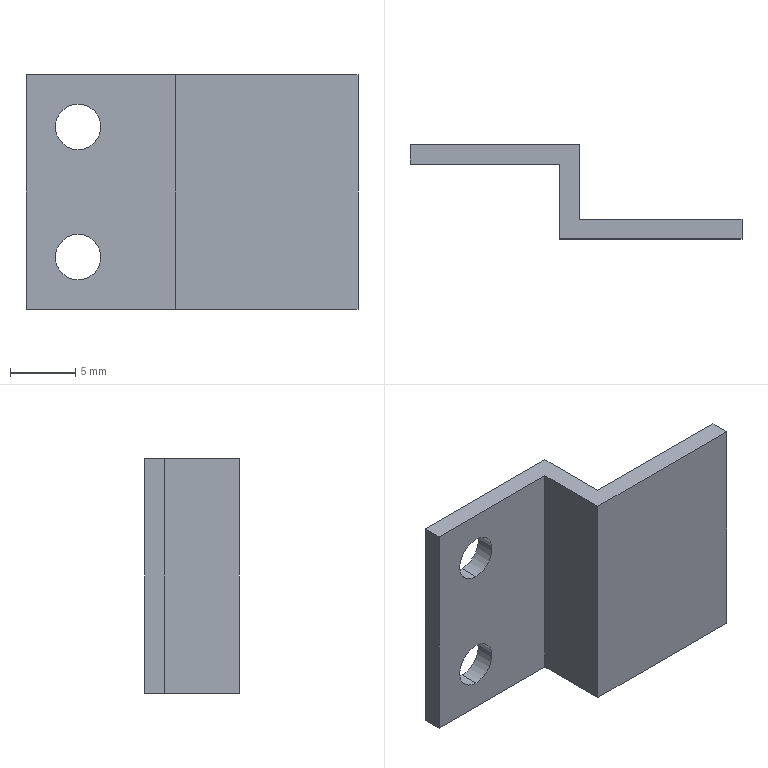Part | STEP file | SM140A-20-1140D-140A-600 External sensor plate | 1 solid | 14 faces | box 25.5 x 7.25 x 18 mm | volume 814.887 mm3 | plane 10 | cylinder 4 | commonest cylinder face diameters 3.5 x4
STEP:
#1=CARTESIAN_POINT('',(0.,0.,0.));
#2=DIRECTION('',(0.,0.,1.));
#3=DIRECTION('',(1.,0.,0.));
#4=AXIS2_PLACEMENT_3D('',#1,#2,#3);
#5=CARTESIAN_POINT('',(4.,-1.5,5.75));
#6=VERTEX_POINT('',#5);
#7=CARTESIAN_POINT('',(4.,0.,5.75));
#8=VERTEX_POINT('',#7);
#9=CARTESIAN_POINT('',(4.,-7.25,5.75));
#10=DIRECTION('',(0.,1.,0.));
#11=VECTOR('',#10,1.);
#12=LINE('',#9,#11);
#13=CARTESIAN_POINT('',(4.,-7.25,4.));
#14=DIRECTION('',(0.,1.,0.));
#15=DIRECTION('',(0.,0.,1.));
#16=AXIS2_PLACEMENT_3D('',#13,#14,#15);
#17=CYLINDRICAL_SURFACE('',#16,1.75);
#18=CARTESIAN_POINT('',(6.283,0.));
#19=DIRECTION('',(0.,1.));
#20=VECTOR('',#19,1.);
#21=LINE('',#18,#20);
#22=(GEOMETRIC_REPRESENTATION_CONTEXT(2)PARAMETRIC_REPRESENTATION_CONTEXT()REPRESENTATION_CONTEXT('',''));
#23=DEFINITIONAL_REPRESENTATION('',(#21),#22);
#24=PCURVE('',#17,#23);
#25=CARTESIAN_POINT('',(4.,-7.25,4.));
#26=DIRECTION('',(0.,1.,0.));
#27=DIRECTION('',(0.,0.,1.));
#28=AXIS2_PLACEMENT_3D('',#25,#26,#27);
#29=CYLINDRICAL_SURFACE('',#28,1.75);
#30=CARTESIAN_POINT('',(0.,0.));
#31=DIRECTION('',(0.,1.));
#32=VECTOR('',#31,1.);
#33=LINE('',#30,#32);
#34=(GEOMETRIC_REPRESENTATION_CONTEXT(2)PARAMETRIC_REPRESENTATION_CONTEXT()REPRESENTATION_CONTEXT('',''));
#35=DEFINITIONAL_REPRESENTATION('',(#33),#34);
#36=PCURVE('',#29,#35);
#37=SURFACE_CURVE('',#12,(#24,#36),.PCURVE_S1.);
#38=EDGE_CURVE('',#6,#8,#37,.T.);
#39=ORIENTED_EDGE('',*,*,#38,.T.);
#40=CARTESIAN_POINT('',(4.,0.,2.25));
#41=VERTEX_POINT('',#40);
#42=CARTESIAN_POINT('',(4.,0.,4.));
#43=DIRECTION('',(0.,1.,0.));
#44=DIRECTION('',(0.,0.,1.));
#45=AXIS2_PLACEMENT_3D('',#42,#43,#44);
#46=CIRCLE('',#45,1.75);
#47=CARTESIAN_POINT('',(0.,7.25));
#48=DIRECTION('',(1.,0.));
#49=VECTOR('',#48,1.);
#50=LINE('',#47,#49);
#51=(GEOMETRIC_REPRESENTATION_CONTEXT(2)PARAMETRIC_REPRESENTATION_CONTEXT()REPRESENTATION_CONTEXT('',''));
#52=DEFINITIONAL_REPRESENTATION('',(#50),#51);
#53=PCURVE('',#17,#52);
#54=CARTESIAN_POINT('',(0.,0.,18.));
#55=DIRECTION('',(0.,-1.,0.));
#56=DIRECTION('',(0.,0.,-1.));
#57=AXIS2_PLACEMENT_3D('',#54,#55,#56);
#58=PLANE('',#57);
#59=CARTESIAN_POINT('',(12.25,4.));
#60=CARTESIAN_POINT('',(12.25,7.031));
#61=CARTESIAN_POINT('',(14.875,5.516));
#62=CARTESIAN_POINT('',(17.5,4.));
#63=CARTESIAN_POINT('',(14.875,2.484));
#64=CARTESIAN_POINT('',(12.25,0.9689));
#65=CARTESIAN_POINT('',(12.25,4.));
#66=(BOUNDED_CURVE()B_SPLINE_CURVE(2,(#59,#60,#61,#62,#63,#64,#65),.UNSPECIFIED.,.T.,.F.)B_SPLINE_CURVE_WITH_KNOTS((1,2,2,2,2,1),(-2.094,0.,2.094,4.189,6.283,8.378),.UNSPECIFIED.)CURVE()GEOMETRIC_REPRESENTATION_ITEM()RATIONAL_B_SPLINE_CURVE((1.,0.5,1.,0.5,1.,0.5,1.))REPRESENTATION_ITEM(''));
#67=(GEOMETRIC_REPRESENTATION_CONTEXT(2)PARAMETRIC_REPRESENTATION_CONTEXT()REPRESENTATION_CONTEXT('',''));
#68=DEFINITIONAL_REPRESENTATION('',(#66),#67);
#69=PCURVE('',#58,#68);
#70=SURFACE_CURVE('',#46,(#53,#69),.PCURVE_S1.);
#71=EDGE_CURVE('',#41,#8,#70,.T.);
#72=ORIENTED_EDGE('',*,*,#71,.F.);
#73=CARTESIAN_POINT('',(4.,-1.5,2.25));
#74=VERTEX_POINT('',#73);
#75=CARTESIAN_POINT('',(4.,-7.25,2.25));
#76=DIRECTION('',(0.,1.,0.));
#77=VECTOR('',#76,1.);
#78=LINE('',#75,#77);
#79=CARTESIAN_POINT('',(3.142,0.));
#80=DIRECTION('',(0.,1.));
#81=VECTOR('',#80,1.);
#82=LINE('',#79,#81);
#83=(GEOMETRIC_REPRESENTATION_CONTEXT(2)PARAMETRIC_REPRESENTATION_CONTEXT()REPRESENTATION_CONTEXT('',''));
#84=DEFINITIONAL_REPRESENTATION('',(#82),#83);
#85=PCURVE('',#17,#84);
#86=CARTESIAN_POINT('',(3.142,0.));
#87=DIRECTION('',(0.,1.));
#88=VECTOR('',#87,1.);
#89=LINE('',#86,#88);
#90=(GEOMETRIC_REPRESENTATION_CONTEXT(2)PARAMETRIC_REPRESENTATION_CONTEXT()REPRESENTATION_CONTEXT('',''));
#91=DEFINITIONAL_REPRESENTATION('',(#89),#90);
#92=PCURVE('',#29,#91);
#93=SURFACE_CURVE('',#78,(#85,#92),.PCURVE_S1.);
#94=EDGE_CURVE('',#74,#41,#93,.T.);
#95=ORIENTED_EDGE('',*,*,#94,.F.);
#96=CARTESIAN_POINT('',(4.,-1.5,4.));
#97=DIRECTION('',(0.,1.,0.));
#98=DIRECTION('',(-1.,0.,0.));
#99=AXIS2_PLACEMENT_3D('',#96,#97,#98);
#100=CIRCLE('',#99,1.75);
#101=CARTESIAN_POINT('',(-1.571,5.75));
#102=DIRECTION('',(1.,0.));
#103=VECTOR('',#102,1.);
#104=LINE('',#101,#103);
#105=(GEOMETRIC_REPRESENTATION_CONTEXT(2)PARAMETRIC_REPRESENTATION_CONTEXT()REPRESENTATION_CONTEXT('',''));
#106=DEFINITIONAL_REPRESENTATION('',(#104),#105);
#107=PCURVE('',#17,#106);
#108=CARTESIAN_POINT('',(11.5,-1.5,18.));
#109=DIRECTION('',(0.,1.,0.));
#110=DIRECTION('',(-1.,0.,0.));
#111=AXIS2_PLACEMENT_3D('',#108,#109,#110);
#112=PLANE('',#111);
#113=CARTESIAN_POINT('',(7.5,-14.));
#114=DIRECTION('',(1.,0.));
#115=AXIS2_PLACEMENT_2D('',#113,#114);
#116=CIRCLE('',#115,1.75);
#117=(GEOMETRIC_REPRESENTATION_CONTEXT(2)PARAMETRIC_REPRESENTATION_CONTEXT()REPRESENTATION_CONTEXT('',''));
#118=DEFINITIONAL_REPRESENTATION('',(#116),#117);
#119=PCURVE('',#112,#118);
#120=SURFACE_CURVE('',#100,(#107,#119),.PCURVE_S1.);
#121=EDGE_CURVE('',#74,#6,#120,.T.);
#122=ORIENTED_EDGE('',*,*,#121,.T.);
#123=EDGE_LOOP('',(#39,#72,#95,#122));
#124=FACE_BOUND('',#123,.F.);
#125=ADVANCED_FACE('',(#124),#17,.F.);
#126=CARTESIAN_POINT('',(4.,-1.5,15.75));
#127=VERTEX_POINT('',#126);
#128=CARTESIAN_POINT('',(4.,0.,15.75));
#129=VERTEX_POINT('',#128);
#130=CARTESIAN_POINT('',(4.,-7.25,15.75));
#131=DIRECTION('',(0.,1.,0.));
#132=VECTOR('',#131,1.);
#133=LINE('',#130,#132);
#134=CARTESIAN_POINT('',(4.,-7.25,14.));
#135=DIRECTION('',(0.,1.,0.));
#136=DIRECTION('',(0.,0.,1.));
#137=AXIS2_PLACEMENT_3D('',#134,#135,#136);
#138=CYLINDRICAL_SURFACE('',#137,1.75);
#139=CARTESIAN_POINT('',(6.283,0.));
#140=DIRECTION('',(0.,1.));
#141=VECTOR('',#140,1.);
#142=LINE('',#139,#141);
#143=(GEOMETRIC_REPRESENTATION_CONTEXT(2)PARAMETRIC_REPRESENTATION_CONTEXT()REPRESENTATION_CONTEXT('',''));
#144=DEFINITIONAL_REPRESENTATION('',(#142),#143);
#145=PCURVE('',#138,#144);
#146=CARTESIAN_POINT('',(4.,-7.25,14.));
#147=DIRECTION('',(0.,1.,0.));
#148=DIRECTION('',(0.,0.,1.));
#149=AXIS2_PLACEMENT_3D('',#146,#147,#148);
#150=CYLINDRICAL_SURFACE('',#149,1.75);
#151=CARTESIAN_POINT('',(0.,0.));
#152=DIRECTION('',(0.,1.));
#153=VECTOR('',#152,1.);
#154=LINE('',#151,#153);
#155=(GEOMETRIC_REPRESENTATION_CONTEXT(2)PARAMETRIC_REPRESENTATION_CONTEXT()REPRESENTATION_CONTEXT('',''));
#156=DEFINITIONAL_REPRESENTATION('',(#154),#155);
#157=PCURVE('',#150,#156);
#158=SURFACE_CURVE('',#133,(#145,#157),.PCURVE_S1.);
#159=EDGE_CURVE('',#127,#129,#158,.T.);
#160=ORIENTED_EDGE('',*,*,#159,.T.);
#161=CARTESIAN_POINT('',(4.,0.,12.25));
#162=VERTEX_POINT('',#161);
#163=CARTESIAN_POINT('',(4.,0.,14.));
#164=DIRECTION('',(0.,1.,0.));
#165=DIRECTION('',(0.,0.,1.));
#166=AXIS2_PLACEMENT_3D('',#163,#164,#165);
#167=CIRCLE('',#166,1.75);
#168=CARTESIAN_POINT('',(0.,7.25));
#169=DIRECTION('',(1.,0.));
#170=VECTOR('',#169,1.);
#171=LINE('',#168,#170);
#172=(GEOMETRIC_REPRESENTATION_CONTEXT(2)PARAMETRIC_REPRESENTATION_CONTEXT()REPRESENTATION_CONTEXT('',''));
#173=DEFINITIONAL_REPRESENTATION('',(#171),#172);
#174=PCURVE('',#138,#173);
#175=CARTESIAN_POINT('',(2.25,4.));
#176=CARTESIAN_POINT('',(2.25,7.031));
#177=CARTESIAN_POINT('',(4.875,5.516));
#178=CARTESIAN_POINT('',(7.5,4.));
#179=CARTESIAN_POINT('',(4.875,2.484));
#180=CARTESIAN_POINT('',(2.25,0.9689));
#181=CARTESIAN_POINT('',(2.25,4.));
#182=(BOUNDED_CURVE()B_SPLINE_CURVE(2,(#175,#176,#177,#178,#179,#180,#181),.UNSPECIFIED.,.T.,.F.)B_SPLINE_CURVE_WITH_KNOTS((1,2,2,2,2,1),(-2.094,0.,2.094,4.189,6.283,8.378),.UNSPECIFIED.)CURVE()GEOMETRIC_REPRESENTATION_ITEM()RATIONAL_B_SPLINE_CURVE((1.,0.5,1.,0.5,1.,0.5,1.))REPRESENTATION_ITEM(''));
#183=(GEOMETRIC_REPRESENTATION_CONTEXT(2)PARAMETRIC_REPRESENTATION_CONTEXT()REPRESENTATION_CONTEXT('',''));
#184=DEFINITIONAL_REPRESENTATION('',(#182),#183);
#185=PCURVE('',#58,#184);
#186=SURFACE_CURVE('',#167,(#174,#185),.PCURVE_S1.);
#187=EDGE_CURVE('',#162,#129,#186,.T.);
#188=ORIENTED_EDGE('',*,*,#187,.F.);
#189=CARTESIAN_POINT('',(4.,-1.5,12.25));
#190=VERTEX_POINT('',#189);
#191=CARTESIAN_POINT('',(4.,-7.25,12.25));
#192=DIRECTION('',(0.,1.,0.));
#193=VECTOR('',#192,1.);
#194=LINE('',#191,#193);
#195=CARTESIAN_POINT('',(3.142,0.));
#196=DIRECTION('',(0.,1.));
#197=VECTOR('',#196,1.);
#198=LINE('',#195,#197);
#199=(GEOMETRIC_REPRESENTATION_CONTEXT(2)PARAMETRIC_REPRESENTATION_CONTEXT()REPRESENTATION_CONTEXT('',''));
#200=DEFINITIONAL_REPRESENTATION('',(#198),#199);
#201=PCURVE('',#138,#200);
#202=CARTESIAN_POINT('',(3.142,0.));
#203=DIRECTION('',(0.,1.));
#204=VECTOR('',#203,1.);
#205=LINE('',#202,#204);
#206=(GEOMETRIC_REPRESENTATION_CONTEXT(2)PARAMETRIC_REPRESENTATION_CONTEXT()REPRESENTATION_CONTEXT('',''));
#207=DEFINITIONAL_REPRESENTATION('',(#205),#206);
#208=PCURVE('',#150,#207);
#209=SURFACE_CURVE('',#194,(#201,#208),.PCURVE_S1.);
#210=EDGE_CURVE('',#190,#162,#209,.T.);
#211=ORIENTED_EDGE('',*,*,#210,.F.);
#212=CARTESIAN_POINT('',(4.,-1.5,14.));
#213=DIRECTION('',(0.,1.,0.));
#214=DIRECTION('',(-1.,0.,0.));
#215=AXIS2_PLACEMENT_3D('',#212,#213,#214);
#216=CIRCLE('',#215,1.75);
#217=CARTESIAN_POINT('',(-1.571,5.75));
#218=DIRECTION('',(1.,0.));
#219=VECTOR('',#218,1.);
#220=LINE('',#217,#219);
#221=(GEOMETRIC_REPRESENTATION_CONTEXT(2)PARAMETRIC_REPRESENTATION_CONTEXT()REPRESENTATION_CONTEXT('',''));
#222=DEFINITIONAL_REPRESENTATION('',(#220),#221);
#223=PCURVE('',#138,#222);
#224=CARTESIAN_POINT('',(7.5,-4.));
#225=DIRECTION('',(1.,0.));
#226=AXIS2_PLACEMENT_2D('',#224,#225);
#227=CIRCLE('',#226,1.75);
#228=(GEOMETRIC_REPRESENTATION_CONTEXT(2)PARAMETRIC_REPRESENTATION_CONTEXT()REPRESENTATION_CONTEXT('',''));
#229=DEFINITIONAL_REPRESENTATION('',(#227),#228);
#230=PCURVE('',#112,#229);
#231=SURFACE_CURVE('',#216,(#223,#230),.PCURVE_S1.);
#232=EDGE_CURVE('',#190,#127,#231,.T.);
#233=ORIENTED_EDGE('',*,*,#232,.T.);
#234=EDGE_LOOP('',(#160,#188,#211,#233));
#235=FACE_BOUND('',#234,.F.);
#236=ADVANCED_FACE('',(#235),#138,.F.);
#237=CARTESIAN_POINT('',(0.,0.,0.));
#238=VERTEX_POINT('',#237);
#239=CARTESIAN_POINT('',(0.,-1.5,0.));
#240=VERTEX_POINT('',#239);
#241=CARTESIAN_POINT('',(0.,-1.5,0.));
#242=DIRECTION('',(0.,-1.,0.));
#243=VECTOR('',#242,1.);
#244=LINE('',#241,#243);
#245=CARTESIAN_POINT('',(0.,-1.5,18.));
#246=DIRECTION('',(1.,0.,0.));
#247=DIRECTION('',(0.,0.,-1.));
#248=AXIS2_PLACEMENT_3D('',#245,#246,#247);
#249=PLANE('',#248);
#250=CARTESIAN_POINT('',(18.,0.));
#251=DIRECTION('',(0.,-1.));
#252=VECTOR('',#251,1.);
#253=LINE('',#250,#252);
#254=(GEOMETRIC_REPRESENTATION_CONTEXT(2)PARAMETRIC_REPRESENTATION_CONTEXT()REPRESENTATION_CONTEXT('',''));
#255=DEFINITIONAL_REPRESENTATION('',(#253),#254);
#256=PCURVE('',#249,#255);
#257=CARTESIAN_POINT('',(0.,0.,0.));
#258=DIRECTION('',(0.,0.,-1.));
#259=DIRECTION('',(-1.,0.,0.));
#260=AXIS2_PLACEMENT_3D('',#257,#258,#259);
#261=PLANE('',#260);
#262=CARTESIAN_POINT('',(0.,-1.5));
#263=DIRECTION('',(0.,-1.));
#264=VECTOR('',#263,1.);
#265=LINE('',#262,#264);
#266=(GEOMETRIC_REPRESENTATION_CONTEXT(2)PARAMETRIC_REPRESENTATION_CONTEXT()REPRESENTATION_CONTEXT('',''));
#267=DEFINITIONAL_REPRESENTATION('',(#265),#266);
#268=PCURVE('',#261,#267);
#269=SURFACE_CURVE('',#244,(#256,#268),.PCURVE_S1.);
#270=EDGE_CURVE('',#238,#240,#269,.T.);
#271=ORIENTED_EDGE('',*,*,#270,.T.);
#272=CARTESIAN_POINT('',(0.,-1.5,18.));
#273=VERTEX_POINT('',#272);
#274=CARTESIAN_POINT('',(0.,-1.5,18.));
#275=DIRECTION('',(0.,0.,-1.));
#276=VECTOR('',#275,1.);
#277=LINE('',#274,#276);
#278=CARTESIAN_POINT('',(0.,0.));
#279=DIRECTION('',(1.,0.));
#280=VECTOR('',#279,1.);
#281=LINE('',#278,#280);
#282=(GEOMETRIC_REPRESENTATION_CONTEXT(2)PARAMETRIC_REPRESENTATION_CONTEXT()REPRESENTATION_CONTEXT('',''));
#283=DEFINITIONAL_REPRESENTATION('',(#281),#282);
#284=PCURVE('',#249,#283);
#285=CARTESIAN_POINT('',(11.5,0.));
#286=DIRECTION('',(0.,-1.));
#287=VECTOR('',#286,1.);
#288=LINE('',#285,#287);
#289=(GEOMETRIC_REPRESENTATION_CONTEXT(2)PARAMETRIC_REPRESENTATION_CONTEXT()REPRESENTATION_CONTEXT('',''));
#290=DEFINITIONAL_REPRESENTATION('',(#288),#289);
#291=PCURVE('',#112,#290);
#292=SURFACE_CURVE('',#277,(#284,#291),.PCURVE_S1.);
#293=EDGE_CURVE('',#273,#240,#292,.T.);
#294=ORIENTED_EDGE('',*,*,#293,.F.);
#295=CARTESIAN_POINT('',(0.,0.,18.));
#296=VERTEX_POINT('',#295);
#297=CARTESIAN_POINT('',(0.,-1.5,18.));
#298=DIRECTION('',(0.,-1.,0.));
#299=VECTOR('',#298,1.);
#300=LINE('',#297,#299);
#301=CARTESIAN_POINT('',(0.,0.));
#302=DIRECTION('',(0.,-1.));
#303=VECTOR('',#302,1.);
#304=LINE('',#301,#303);
#305=(GEOMETRIC_REPRESENTATION_CONTEXT(2)PARAMETRIC_REPRESENTATION_CONTEXT()REPRESENTATION_CONTEXT('',''));
#306=DEFINITIONAL_REPRESENTATION('',(#304),#305);
#307=PCURVE('',#249,#306);
#308=CARTESIAN_POINT('',(0.,0.,18.));
#309=DIRECTION('',(0.,0.,-1.));
#310=DIRECTION('',(-1.,0.,0.));
#311=AXIS2_PLACEMENT_3D('',#308,#309,#310);
#312=PLANE('',#311);
#313=CARTESIAN_POINT('',(0.,-1.5));
#314=DIRECTION('',(0.,-1.));
#315=VECTOR('',#314,1.);
#316=LINE('',#313,#315);
#317=(GEOMETRIC_REPRESENTATION_CONTEXT(2)PARAMETRIC_REPRESENTATION_CONTEXT()REPRESENTATION_CONTEXT('',''));
#318=DEFINITIONAL_REPRESENTATION('',(#316),#317);
#319=PCURVE('',#312,#318);
#320=SURFACE_CURVE('',#300,(#307,#319),.PCURVE_S1.);
#321=EDGE_CURVE('',#296,#273,#320,.T.);
#322=ORIENTED_EDGE('',*,*,#321,.F.);
#323=CARTESIAN_POINT('',(0.,0.,18.));
#324=DIRECTION('',(0.,0.,-1.));
#325=VECTOR('',#324,1.);
#326=LINE('',#323,#325);
#327=CARTESIAN_POINT('',(0.,1.5));
#328=DIRECTION('',(1.,0.));
#329=VECTOR('',#328,1.);
#330=LINE('',#327,#329);
#331=(GEOMETRIC_REPRESENTATION_CONTEXT(2)PARAMETRIC_REPRESENTATION_CONTEXT()REPRESENTATION_CONTEXT('',''));
#332=DEFINITIONAL_REPRESENTATION('',(#330),#331);
#333=PCURVE('',#249,#332);
#334=CARTESIAN_POINT('',(0.,0.));
#335=DIRECTION('',(1.,0.));
#336=VECTOR('',#335,1.);
#337=LINE('',#334,#336);
#338=(GEOMETRIC_REPRESENTATION_CONTEXT(2)PARAMETRIC_REPRESENTATION_CONTEXT()REPRESENTATION_CONTEXT('',''));
#339=DEFINITIONAL_REPRESENTATION('',(#337),#338);
#340=PCURVE('',#58,#339);
#341=SURFACE_CURVE('',#326,(#333,#340),.PCURVE_S1.);
#342=EDGE_CURVE('',#296,#238,#341,.T.);
#343=ORIENTED_EDGE('',*,*,#342,.T.);
#344=EDGE_LOOP('',(#271,#294,#322,#343));
#345=FACE_BOUND('',#344,.T.);
#346=ADVANCED_FACE('',(#345),#249,.F.);
#347=CARTESIAN_POINT('',(4.,-1.5,4.));
#348=DIRECTION('',(0.,1.,0.));
#349=DIRECTION('',(-1.,0.,0.));
#350=AXIS2_PLACEMENT_3D('',#347,#348,#349);
#351=CIRCLE('',#350,1.75);
#352=CARTESIAN_POINT('',(7.5,-14.));
#353=DIRECTION('',(1.,0.));
#354=AXIS2_PLACEMENT_2D('',#352,#353);
#355=CIRCLE('',#354,1.75);
#356=(GEOMETRIC_REPRESENTATION_CONTEXT(2)PARAMETRIC_REPRESENTATION_CONTEXT()REPRESENTATION_CONTEXT('',''));
#357=DEFINITIONAL_REPRESENTATION('',(#355),#356);
#358=PCURVE('',#112,#357);
#359=CARTESIAN_POINT('',(-1.571,5.75));
#360=DIRECTION('',(1.,0.));
#361=VECTOR('',#360,1.);
#362=LINE('',#359,#361);
#363=(GEOMETRIC_REPRESENTATION_CONTEXT(2)PARAMETRIC_REPRESENTATION_CONTEXT()REPRESENTATION_CONTEXT('',''));
#364=DEFINITIONAL_REPRESENTATION('',(#362),#363);
#365=PCURVE('',#29,#364);
#366=SURFACE_CURVE('',#351,(#358,#365),.PCURVE_S1.);
#367=EDGE_CURVE('',#6,#74,#366,.T.);
#368=ORIENTED_EDGE('',*,*,#367,.T.);
#369=ORIENTED_EDGE('',*,*,#121,.T.);
#370=EDGE_LOOP('',(#368,#369));
#371=FACE_BOUND('',#370,.T.);
#372=CARTESIAN_POINT('',(4.,-1.5,14.));
#373=DIRECTION('',(0.,1.,0.));
#374=DIRECTION('',(-1.,0.,0.));
#375=AXIS2_PLACEMENT_3D('',#372,#373,#374);
#376=CIRCLE('',#375,1.75);
#377=CARTESIAN_POINT('',(7.5,-4.));
#378=DIRECTION('',(1.,0.));
#379=AXIS2_PLACEMENT_2D('',#377,#378);
#380=CIRCLE('',#379,1.75);
#381=(GEOMETRIC_REPRESENTATION_CONTEXT(2)PARAMETRIC_REPRESENTATION_CONTEXT()REPRESENTATION_CONTEXT('',''));
#382=DEFINITIONAL_REPRESENTATION('',(#380),#381);
#383=PCURVE('',#112,#382);
#384=CARTESIAN_POINT('',(-1.571,5.75));
#385=DIRECTION('',(1.,0.));
#386=VECTOR('',#385,1.);
#387=LINE('',#384,#386);
#388=(GEOMETRIC_REPRESENTATION_CONTEXT(2)PARAMETRIC_REPRESENTATION_CONTEXT()REPRESENTATION_CONTEXT('',''));
#389=DEFINITIONAL_REPRESENTATION('',(#387),#388);
#390=PCURVE('',#150,#389);
#391=SURFACE_CURVE('',#376,(#383,#390),.PCURVE_S1.);
#392=EDGE_CURVE('',#127,#190,#391,.T.);
#393=ORIENTED_EDGE('',*,*,#392,.T.);
#394=ORIENTED_EDGE('',*,*,#232,.T.);
#395=EDGE_LOOP('',(#393,#394));
#396=FACE_BOUND('',#395,.T.);
#397=CARTESIAN_POINT('',(11.5,-1.5,0.));
#398=VERTEX_POINT('',#397);
#399=CARTESIAN_POINT('',(11.5,-1.5,0.));
#400=DIRECTION('',(1.,0.,0.));
#401=VECTOR('',#400,1.);
#402=LINE('',#399,#401);
#403=CARTESIAN_POINT('',(0.,-18.));
#404=DIRECTION('',(-1.,0.));
#405=VECTOR('',#404,1.);
#406=LINE('',#403,#405);
#407=(GEOMETRIC_REPRESENTATION_CONTEXT(2)PARAMETRIC_REPRESENTATION_CONTEXT()REPRESENTATION_CONTEXT('',''));
#408=DEFINITIONAL_REPRESENTATION('',(#406),#407);
#409=PCURVE('',#112,#408);
#410=CARTESIAN_POINT('',(-11.5,-1.5));
#411=DIRECTION('',(-1.,0.));
#412=VECTOR('',#411,1.);
#413=LINE('',#410,#412);
#414=(GEOMETRIC_REPRESENTATION_CONTEXT(2)PARAMETRIC_REPRESENTATION_CONTEXT()REPRESENTATION_CONTEXT('',''));
#415=DEFINITIONAL_REPRESENTATION('',(#413),#414);
#416=PCURVE('',#261,#415);
#417=SURFACE_CURVE('',#402,(#409,#416),.PCURVE_S1.);
#418=EDGE_CURVE('',#240,#398,#417,.T.);
#419=ORIENTED_EDGE('',*,*,#418,.T.);
#420=CARTESIAN_POINT('',(11.5,-1.5,18.));
#421=VERTEX_POINT('',#420);
#422=CARTESIAN_POINT('',(11.5,-1.5,18.));
#423=DIRECTION('',(0.,0.,-1.));
#424=VECTOR('',#423,1.);
#425=LINE('',#422,#424);
#426=CARTESIAN_POINT('',(0.,0.));
#427=DIRECTION('',(0.,-1.));
#428=VECTOR('',#427,1.);
#429=LINE('',#426,#428);
#430=(GEOMETRIC_REPRESENTATION_CONTEXT(2)PARAMETRIC_REPRESENTATION_CONTEXT()REPRESENTATION_CONTEXT('',''));
#431=DEFINITIONAL_REPRESENTATION('',(#429),#430);
#432=PCURVE('',#112,#431);
#433=CARTESIAN_POINT('',(11.5,-7.25,18.));
#434=DIRECTION('',(1.,0.,0.));
#435=DIRECTION('',(0.,0.,-1.));
#436=AXIS2_PLACEMENT_3D('',#433,#434,#435);
#437=PLANE('',#436);
#438=CARTESIAN_POINT('',(0.,5.75));
#439=DIRECTION('',(1.,0.));
#440=VECTOR('',#439,1.);
#441=LINE('',#438,#440);
#442=(GEOMETRIC_REPRESENTATION_CONTEXT(2)PARAMETRIC_REPRESENTATION_CONTEXT()REPRESENTATION_CONTEXT('',''));
#443=DEFINITIONAL_REPRESENTATION('',(#441),#442);
#444=PCURVE('',#437,#443);
#445=SURFACE_CURVE('',#425,(#432,#444),.PCURVE_S1.);
#446=EDGE_CURVE('',#421,#398,#445,.T.);
#447=ORIENTED_EDGE('',*,*,#446,.F.);
#448=CARTESIAN_POINT('',(11.5,-1.5,18.));
#449=DIRECTION('',(1.,0.,0.));
#450=VECTOR('',#449,1.);
#451=LINE('',#448,#450);
#452=CARTESIAN_POINT('',(0.,0.));
#453=DIRECTION('',(-1.,0.));
#454=VECTOR('',#453,1.);
#455=LINE('',#452,#454);
#456=(GEOMETRIC_REPRESENTATION_CONTEXT(2)PARAMETRIC_REPRESENTATION_CONTEXT()REPRESENTATION_CONTEXT('',''));
#457=DEFINITIONAL_REPRESENTATION('',(#455),#456);
#458=PCURVE('',#112,#457);
#459=CARTESIAN_POINT('',(-11.5,-1.5));
#460=DIRECTION('',(-1.,0.));
#461=VECTOR('',#460,1.);
#462=LINE('',#459,#461);
#463=(GEOMETRIC_REPRESENTATION_CONTEXT(2)PARAMETRIC_REPRESENTATION_CONTEXT()REPRESENTATION_CONTEXT('',''));
#464=DEFINITIONAL_REPRESENTATION('',(#462),#463);
#465=PCURVE('',#312,#464);
#466=SURFACE_CURVE('',#451,(#458,#465),.PCURVE_S1.);
#467=EDGE_CURVE('',#273,#421,#466,.T.);
#468=ORIENTED_EDGE('',*,*,#467,.F.);
#469=ORIENTED_EDGE('',*,*,#293,.T.);
#470=EDGE_LOOP('',(#419,#447,#468,#469));
#471=FACE_BOUND('',#470,.T.);
#472=ADVANCED_FACE('',(#371,#396,#471),#112,.F.);
#473=CARTESIAN_POINT('',(11.5,-7.25,0.));
#474=VERTEX_POINT('',#473);
#475=CARTESIAN_POINT('',(11.5,-7.25,0.));
#476=DIRECTION('',(0.,-1.,0.));
#477=VECTOR('',#476,1.);
#478=LINE('',#475,#477);
#479=CARTESIAN_POINT('',(18.,0.));
#480=DIRECTION('',(0.,-1.));
#481=VECTOR('',#480,1.);
#482=LINE('',#479,#481);
#483=(GEOMETRIC_REPRESENTATION_CONTEXT(2)PARAMETRIC_REPRESENTATION_CONTEXT()REPRESENTATION_CONTEXT('',''));
#484=DEFINITIONAL_REPRESENTATION('',(#482),#483);
#485=PCURVE('',#437,#484);
#486=CARTESIAN_POINT('',(-11.5,-7.25));
#487=DIRECTION('',(0.,-1.));
#488=VECTOR('',#487,1.);
#489=LINE('',#486,#488);
#490=(GEOMETRIC_REPRESENTATION_CONTEXT(2)PARAMETRIC_REPRESENTATION_CONTEXT()REPRESENTATION_CONTEXT('',''));
#491=DEFINITIONAL_REPRESENTATION('',(#489),#490);
#492=PCURVE('',#261,#491);
#493=SURFACE_CURVE('',#478,(#485,#492),.PCURVE_S1.);
#494=EDGE_CURVE('',#398,#474,#493,.T.);
#495=ORIENTED_EDGE('',*,*,#494,.T.);
#496=CARTESIAN_POINT('',(11.5,-7.25,18.));
#497=VERTEX_POINT('',#496);
#498=CARTESIAN_POINT('',(11.5,-7.25,18.));
#499=DIRECTION('',(0.,0.,-1.));
#500=VECTOR('',#499,1.);
#501=LINE('',#498,#500);
#502=CARTESIAN_POINT('',(0.,0.));
#503=DIRECTION('',(1.,0.));
#504=VECTOR('',#503,1.);
#505=LINE('',#502,#504);
#506=(GEOMETRIC_REPRESENTATION_CONTEXT(2)PARAMETRIC_REPRESENTATION_CONTEXT()REPRESENTATION_CONTEXT('',''));
#507=DEFINITIONAL_REPRESENTATION('',(#505),#506);
#508=PCURVE('',#437,#507);
#509=CARTESIAN_POINT('',(25.5,-7.25,18.));
#510=DIRECTION('',(0.,1.,0.));
#511=DIRECTION('',(-1.,0.,0.));
#512=AXIS2_PLACEMENT_3D('',#509,#510,#511);
#513=PLANE('',#512);
#514=CARTESIAN_POINT('',(14.,0.));
#515=DIRECTION('',(0.,-1.));
#516=VECTOR('',#515,1.);
#517=LINE('',#514,#516);
#518=(GEOMETRIC_REPRESENTATION_CONTEXT(2)PARAMETRIC_REPRESENTATION_CONTEXT()REPRESENTATION_CONTEXT('',''));
#519=DEFINITIONAL_REPRESENTATION('',(#517),#518);
#520=PCURVE('',#513,#519);
#521=SURFACE_CURVE('',#501,(#508,#520),.PCURVE_S1.);
#522=EDGE_CURVE('',#497,#474,#521,.T.);
#523=ORIENTED_EDGE('',*,*,#522,.F.);
#524=CARTESIAN_POINT('',(11.5,-7.25,18.));
#525=DIRECTION('',(0.,-1.,0.));
#526=VECTOR('',#525,1.);
#527=LINE('',#524,#526);
#528=CARTESIAN_POINT('',(0.,0.));
#529=DIRECTION('',(0.,-1.));
#530=VECTOR('',#529,1.);
#531=LINE('',#528,#530);
#532=(GEOMETRIC_REPRESENTATION_CONTEXT(2)PARAMETRIC_REPRESENTATION_CONTEXT()REPRESENTATION_CONTEXT('',''));
#533=DEFINITIONAL_REPRESENTATION('',(#531),#532);
#534=PCURVE('',#437,#533);
#535=CARTESIAN_POINT('',(-11.5,-7.25));
#536=DIRECTION('',(0.,-1.));
#537=VECTOR('',#536,1.);
#538=LINE('',#535,#537);
#539=(GEOMETRIC_REPRESENTATION_CONTEXT(2)PARAMETRIC_REPRESENTATION_CONTEXT()REPRESENTATION_CONTEXT('',''));
#540=DEFINITIONAL_REPRESENTATION('',(#538),#539);
#541=PCURVE('',#312,#540);
#542=SURFACE_CURVE('',#527,(#534,#541),.PCURVE_S1.);
#543=EDGE_CURVE('',#421,#497,#542,.T.);
#544=ORIENTED_EDGE('',*,*,#543,.F.);
#545=ORIENTED_EDGE('',*,*,#446,.T.);
#546=EDGE_LOOP('',(#495,#523,#544,#545));
#547=FACE_BOUND('',#546,.T.);
#548=ADVANCED_FACE('',(#547),#437,.F.);
#549=CARTESIAN_POINT('',(25.5,-7.25,0.));
#550=VERTEX_POINT('',#549);
#551=CARTESIAN_POINT('',(25.5,-7.25,0.));
#552=DIRECTION('',(1.,0.,0.));
#553=VECTOR('',#552,1.);
#554=LINE('',#551,#553);
#555=CARTESIAN_POINT('',(0.,-18.));
#556=DIRECTION('',(-1.,0.));
#557=VECTOR('',#556,1.);
#558=LINE('',#555,#557);
#559=(GEOMETRIC_REPRESENTATION_CONTEXT(2)PARAMETRIC_REPRESENTATION_CONTEXT()REPRESENTATION_CONTEXT('',''));
#560=DEFINITIONAL_REPRESENTATION('',(#558),#559);
#561=PCURVE('',#513,#560);
#562=CARTESIAN_POINT('',(-25.5,-7.25));
#563=DIRECTION('',(-1.,0.));
#564=VECTOR('',#563,1.);
#565=LINE('',#562,#564);
#566=(GEOMETRIC_REPRESENTATION_CONTEXT(2)PARAMETRIC_REPRESENTATION_CONTEXT()REPRESENTATION_CONTEXT('',''));
#567=DEFINITIONAL_REPRESENTATION('',(#565),#566);
#568=PCURVE('',#261,#567);
#569=SURFACE_CURVE('',#554,(#561,#568),.PCURVE_S1.);
#570=EDGE_CURVE('',#474,#550,#569,.T.);
#571=ORIENTED_EDGE('',*,*,#570,.T.);
#572=CARTESIAN_POINT('',(25.5,-7.25,18.));
#573=VERTEX_POINT('',#572);
#574=CARTESIAN_POINT('',(25.5,-7.25,18.));
#575=DIRECTION('',(0.,0.,-1.));
#576=VECTOR('',#575,1.);
#577=LINE('',#574,#576);
#578=CARTESIAN_POINT('',(0.,0.));
#579=DIRECTION('',(0.,-1.));
#580=VECTOR('',#579,1.);
#581=LINE('',#578,#580);
#582=(GEOMETRIC_REPRESENTATION_CONTEXT(2)PARAMETRIC_REPRESENTATION_CONTEXT()REPRESENTATION_CONTEXT('',''));
#583=DEFINITIONAL_REPRESENTATION('',(#581),#582);
#584=PCURVE('',#513,#583);
#585=CARTESIAN_POINT('',(25.5,-5.75,18.));
#586=DIRECTION('',(-1.,0.,0.));
#587=DIRECTION('',(0.,0.,1.));
#588=AXIS2_PLACEMENT_3D('',#585,#586,#587);
#589=PLANE('',#588);
#590=CARTESIAN_POINT('',(0.,-1.5));
#591=DIRECTION('',(-1.,0.));
#592=VECTOR('',#591,1.);
#593=LINE('',#590,#592);
#594=(GEOMETRIC_REPRESENTATION_CONTEXT(2)PARAMETRIC_REPRESENTATION_CONTEXT()REPRESENTATION_CONTEXT('',''));
#595=DEFINITIONAL_REPRESENTATION('',(#593),#594);
#596=PCURVE('',#589,#595);
#597=SURFACE_CURVE('',#577,(#584,#596),.PCURVE_S1.);
#598=EDGE_CURVE('',#573,#550,#597,.T.);
#599=ORIENTED_EDGE('',*,*,#598,.F.);
#600=CARTESIAN_POINT('',(25.5,-7.25,18.));
#601=DIRECTION('',(1.,0.,0.));
#602=VECTOR('',#601,1.);
#603=LINE('',#600,#602);
#604=CARTESIAN_POINT('',(0.,0.));
#605=DIRECTION('',(-1.,0.));
#606=VECTOR('',#605,1.);
#607=LINE('',#604,#606);
#608=(GEOMETRIC_REPRESENTATION_CONTEXT(2)PARAMETRIC_REPRESENTATION_CONTEXT()REPRESENTATION_CONTEXT('',''));
#609=DEFINITIONAL_REPRESENTATION('',(#607),#608);
#610=PCURVE('',#513,#609);
#611=CARTESIAN_POINT('',(-25.5,-7.25));
#612=DIRECTION('',(-1.,0.));
#613=VECTOR('',#612,1.);
#614=LINE('',#611,#613);
#615=(GEOMETRIC_REPRESENTATION_CONTEXT(2)PARAMETRIC_REPRESENTATION_CONTEXT()REPRESENTATION_CONTEXT('',''));
#616=DEFINITIONAL_REPRESENTATION('',(#614),#615);
#617=PCURVE('',#312,#616);
#618=SURFACE_CURVE('',#603,(#610,#617),.PCURVE_S1.);
#619=EDGE_CURVE('',#497,#573,#618,.T.);
#620=ORIENTED_EDGE('',*,*,#619,.F.);
#621=ORIENTED_EDGE('',*,*,#522,.T.);
#622=EDGE_LOOP('',(#571,#599,#620,#621));
#623=FACE_BOUND('',#622,.T.);
#624=ADVANCED_FACE('',(#623),#513,.F.);
#625=CARTESIAN_POINT('',(25.5,-5.75,0.));
#626=VERTEX_POINT('',#625);
#627=CARTESIAN_POINT('',(25.5,-5.75,0.));
#628=DIRECTION('',(0.,1.,0.));
#629=VECTOR('',#628,1.);
#630=LINE('',#627,#629);
#631=CARTESIAN_POINT('',(-18.,0.));
#632=DIRECTION('',(0.,1.));
#633=VECTOR('',#632,1.);
#634=LINE('',#631,#633);
#635=(GEOMETRIC_REPRESENTATION_CONTEXT(2)PARAMETRIC_REPRESENTATION_CONTEXT()REPRESENTATION_CONTEXT('',''));
#636=DEFINITIONAL_REPRESENTATION('',(#634),#635);
#637=PCURVE('',#589,#636);
#638=CARTESIAN_POINT('',(-25.5,-5.75));
#639=DIRECTION('',(0.,1.));
#640=VECTOR('',#639,1.);
#641=LINE('',#638,#640);
#642=(GEOMETRIC_REPRESENTATION_CONTEXT(2)PARAMETRIC_REPRESENTATION_CONTEXT()REPRESENTATION_CONTEXT('',''));
#643=DEFINITIONAL_REPRESENTATION('',(#641),#642);
#644=PCURVE('',#261,#643);
#645=SURFACE_CURVE('',#630,(#637,#644),.PCURVE_S1.);
#646=EDGE_CURVE('',#550,#626,#645,.T.);
#647=ORIENTED_EDGE('',*,*,#646,.T.);
#648=CARTESIAN_POINT('',(25.5,-5.75,18.));
#649=VERTEX_POINT('',#648);
#650=CARTESIAN_POINT('',(25.5,-5.75,18.));
#651=DIRECTION('',(0.,0.,-1.));
#652=VECTOR('',#651,1.);
#653=LINE('',#650,#652);
#654=CARTESIAN_POINT('',(0.,0.));
#655=DIRECTION('',(-1.,0.));
#656=VECTOR('',#655,1.);
#657=LINE('',#654,#656);
#658=(GEOMETRIC_REPRESENTATION_CONTEXT(2)PARAMETRIC_REPRESENTATION_CONTEXT()REPRESENTATION_CONTEXT('',''));
#659=DEFINITIONAL_REPRESENTATION('',(#657),#658);
#660=PCURVE('',#589,#659);
#661=CARTESIAN_POINT('',(13.,-5.75,18.));
#662=DIRECTION('',(0.,-1.,0.));
#663=DIRECTION('',(0.,0.,-1.));
#664=AXIS2_PLACEMENT_3D('',#661,#662,#663);
#665=PLANE('',#664);
#666=CARTESIAN_POINT('',(0.,12.5));
#667=DIRECTION('',(1.,0.));
#668=VECTOR('',#667,1.);
#669=LINE('',#666,#668);
#670=(GEOMETRIC_REPRESENTATION_CONTEXT(2)PARAMETRIC_REPRESENTATION_CONTEXT()REPRESENTATION_CONTEXT('',''));
#671=DEFINITIONAL_REPRESENTATION('',(#669),#670);
#672=PCURVE('',#665,#671);
#673=SURFACE_CURVE('',#653,(#660,#672),.PCURVE_S1.);
#674=EDGE_CURVE('',#649,#626,#673,.T.);
#675=ORIENTED_EDGE('',*,*,#674,.F.);
#676=CARTESIAN_POINT('',(25.5,-5.75,18.));
#677=DIRECTION('',(0.,1.,0.));
#678=VECTOR('',#677,1.);
#679=LINE('',#676,#678);
#680=CARTESIAN_POINT('',(0.,0.));
#681=DIRECTION('',(0.,1.));
#682=VECTOR('',#681,1.);
#683=LINE('',#680,#682);
#684=(GEOMETRIC_REPRESENTATION_CONTEXT(2)PARAMETRIC_REPRESENTATION_CONTEXT()REPRESENTATION_CONTEXT('',''));
#685=DEFINITIONAL_REPRESENTATION('',(#683),#684);
#686=PCURVE('',#589,#685);
#687=CARTESIAN_POINT('',(-25.5,-5.75));
#688=DIRECTION('',(0.,1.));
#689=VECTOR('',#688,1.);
#690=LINE('',#687,#689);
#691=(GEOMETRIC_REPRESENTATION_CONTEXT(2)PARAMETRIC_REPRESENTATION_CONTEXT()REPRESENTATION_CONTEXT('',''));
#692=DEFINITIONAL_REPRESENTATION('',(#690),#691);
#693=PCURVE('',#312,#692);
#694=SURFACE_CURVE('',#679,(#686,#693),.PCURVE_S1.);
#695=EDGE_CURVE('',#573,#649,#694,.T.);
#696=ORIENTED_EDGE('',*,*,#695,.F.);
#697=ORIENTED_EDGE('',*,*,#598,.T.);
#698=EDGE_LOOP('',(#647,#675,#696,#697));
#699=FACE_BOUND('',#698,.T.);
#700=ADVANCED_FACE('',(#699),#589,.F.);
#701=CARTESIAN_POINT('',(13.,-5.75,0.));
#702=VERTEX_POINT('',#701);
#703=CARTESIAN_POINT('',(13.,-5.75,0.));
#704=DIRECTION('',(-1.,0.,0.));
#705=VECTOR('',#704,1.);
#706=LINE('',#703,#705);
#707=CARTESIAN_POINT('',(18.,0.));
#708=DIRECTION('',(0.,-1.));
#709=VECTOR('',#708,1.);
#710=LINE('',#707,#709);
#711=(GEOMETRIC_REPRESENTATION_CONTEXT(2)PARAMETRIC_REPRESENTATION_CONTEXT()REPRESENTATION_CONTEXT('',''));
#712=DEFINITIONAL_REPRESENTATION('',(#710),#711);
#713=PCURVE('',#665,#712);
#714=CARTESIAN_POINT('',(-13.,-5.75));
#715=DIRECTION('',(1.,0.));
#716=VECTOR('',#715,1.);
#717=LINE('',#714,#716);
#718=(GEOMETRIC_REPRESENTATION_CONTEXT(2)PARAMETRIC_REPRESENTATION_CONTEXT()REPRESENTATION_CONTEXT('',''));
#719=DEFINITIONAL_REPRESENTATION('',(#717),#718);
#720=PCURVE('',#261,#719);
#721=SURFACE_CURVE('',#706,(#713,#720),.PCURVE_S1.);
#722=EDGE_CURVE('',#626,#702,#721,.T.);
#723=ORIENTED_EDGE('',*,*,#722,.T.);
#724=CARTESIAN_POINT('',(13.,-5.75,18.));
#725=VERTEX_POINT('',#724);
#726=CARTESIAN_POINT('',(13.,-5.75,18.));
#727=DIRECTION('',(0.,0.,-1.));
#728=VECTOR('',#727,1.);
#729=LINE('',#726,#728);
#730=CARTESIAN_POINT('',(0.,0.));
#731=DIRECTION('',(1.,0.));
#732=VECTOR('',#731,1.);
#733=LINE('',#730,#732);
#734=(GEOMETRIC_REPRESENTATION_CONTEXT(2)PARAMETRIC_REPRESENTATION_CONTEXT()REPRESENTATION_CONTEXT('',''));
#735=DEFINITIONAL_REPRESENTATION('',(#733),#734);
#736=PCURVE('',#665,#735);
#737=CARTESIAN_POINT('',(13.,0.,18.));
#738=DIRECTION('',(-1.,0.,0.));
#739=DIRECTION('',(0.,0.,1.));
#740=AXIS2_PLACEMENT_3D('',#737,#738,#739);
#741=PLANE('',#740);
#742=CARTESIAN_POINT('',(0.,-5.75));
#743=DIRECTION('',(-1.,0.));
#744=VECTOR('',#743,1.);
#745=LINE('',#742,#744);
#746=(GEOMETRIC_REPRESENTATION_CONTEXT(2)PARAMETRIC_REPRESENTATION_CONTEXT()REPRESENTATION_CONTEXT('',''));
#747=DEFINITIONAL_REPRESENTATION('',(#745),#746);
#748=PCURVE('',#741,#747);
#749=SURFACE_CURVE('',#729,(#736,#748),.PCURVE_S1.);
#750=EDGE_CURVE('',#725,#702,#749,.T.);
#751=ORIENTED_EDGE('',*,*,#750,.F.);
#752=CARTESIAN_POINT('',(13.,-5.75,18.));
#753=DIRECTION('',(-1.,0.,0.));
#754=VECTOR('',#753,1.);
#755=LINE('',#752,#754);
#756=CARTESIAN_POINT('',(0.,0.));
#757=DIRECTION('',(0.,-1.));
#758=VECTOR('',#757,1.);
#759=LINE('',#756,#758);
#760=(GEOMETRIC_REPRESENTATION_CONTEXT(2)PARAMETRIC_REPRESENTATION_CONTEXT()REPRESENTATION_CONTEXT('',''));
#761=DEFINITIONAL_REPRESENTATION('',(#759),#760);
#762=PCURVE('',#665,#761);
#763=CARTESIAN_POINT('',(-13.,-5.75));
#764=DIRECTION('',(1.,0.));
#765=VECTOR('',#764,1.);
#766=LINE('',#763,#765);
#767=(GEOMETRIC_REPRESENTATION_CONTEXT(2)PARAMETRIC_REPRESENTATION_CONTEXT()REPRESENTATION_CONTEXT('',''));
#768=DEFINITIONAL_REPRESENTATION('',(#766),#767);
#769=PCURVE('',#312,#768);
#770=SURFACE_CURVE('',#755,(#762,#769),.PCURVE_S1.);
#771=EDGE_CURVE('',#649,#725,#770,.T.);
#772=ORIENTED_EDGE('',*,*,#771,.F.);
#773=ORIENTED_EDGE('',*,*,#674,.T.);
#774=EDGE_LOOP('',(#723,#751,#772,#773));
#775=FACE_BOUND('',#774,.T.);
#776=ADVANCED_FACE('',(#775),#665,.F.);
#777=CARTESIAN_POINT('',(13.,0.,0.));
#778=VERTEX_POINT('',#777);
#779=CARTESIAN_POINT('',(13.,0.,0.));
#780=DIRECTION('',(0.,1.,0.));
#781=VECTOR('',#780,1.);
#782=LINE('',#779,#781);
#783=CARTESIAN_POINT('',(-18.,0.));
#784=DIRECTION('',(0.,1.));
#785=VECTOR('',#784,1.);
#786=LINE('',#783,#785);
#787=(GEOMETRIC_REPRESENTATION_CONTEXT(2)PARAMETRIC_REPRESENTATION_CONTEXT()REPRESENTATION_CONTEXT('',''));
#788=DEFINITIONAL_REPRESENTATION('',(#786),#787);
#789=PCURVE('',#741,#788);
#790=CARTESIAN_POINT('',(-13.,0.));
#791=DIRECTION('',(0.,1.));
#792=VECTOR('',#791,1.);
#793=LINE('',#790,#792);
#794=(GEOMETRIC_REPRESENTATION_CONTEXT(2)PARAMETRIC_REPRESENTATION_CONTEXT()REPRESENTATION_CONTEXT('',''));
#795=DEFINITIONAL_REPRESENTATION('',(#793),#794);
#796=PCURVE('',#261,#795);
#797=SURFACE_CURVE('',#782,(#789,#796),.PCURVE_S1.);
#798=EDGE_CURVE('',#702,#778,#797,.T.);
#799=ORIENTED_EDGE('',*,*,#798,.T.);
#800=CARTESIAN_POINT('',(13.,0.,18.));
#801=VERTEX_POINT('',#800);
#802=CARTESIAN_POINT('',(13.,0.,18.));
#803=DIRECTION('',(0.,0.,-1.));
#804=VECTOR('',#803,1.);
#805=LINE('',#802,#804);
#806=CARTESIAN_POINT('',(0.,0.));
#807=DIRECTION('',(-1.,0.));
#808=VECTOR('',#807,1.);
#809=LINE('',#806,#808);
#810=(GEOMETRIC_REPRESENTATION_CONTEXT(2)PARAMETRIC_REPRESENTATION_CONTEXT()REPRESENTATION_CONTEXT('',''));
#811=DEFINITIONAL_REPRESENTATION('',(#809),#810);
#812=PCURVE('',#741,#811);
#813=CARTESIAN_POINT('',(0.,13.));
#814=DIRECTION('',(1.,0.));
#815=VECTOR('',#814,1.);
#816=LINE('',#813,#815);
#817=(GEOMETRIC_REPRESENTATION_CONTEXT(2)PARAMETRIC_REPRESENTATION_CONTEXT()REPRESENTATION_CONTEXT('',''));
#818=DEFINITIONAL_REPRESENTATION('',(#816),#817);
#819=PCURVE('',#58,#818);
#820=SURFACE_CURVE('',#805,(#812,#819),.PCURVE_S1.);
#821=EDGE_CURVE('',#801,#778,#820,.T.);
#822=ORIENTED_EDGE('',*,*,#821,.F.);
#823=CARTESIAN_POINT('',(13.,0.,18.));
#824=DIRECTION('',(0.,1.,0.));
#825=VECTOR('',#824,1.);
#826=LINE('',#823,#825);
#827=CARTESIAN_POINT('',(0.,0.));
#828=DIRECTION('',(0.,1.));
#829=VECTOR('',#828,1.);
#830=LINE('',#827,#829);
#831=(GEOMETRIC_REPRESENTATION_CONTEXT(2)PARAMETRIC_REPRESENTATION_CONTEXT()REPRESENTATION_CONTEXT('',''));
#832=DEFINITIONAL_REPRESENTATION('',(#830),#831);
#833=PCURVE('',#741,#832);
#834=CARTESIAN_POINT('',(-13.,0.));
#835=DIRECTION('',(0.,1.));
#836=VECTOR('',#835,1.);
#837=LINE('',#834,#836);
#838=(GEOMETRIC_REPRESENTATION_CONTEXT(2)PARAMETRIC_REPRESENTATION_CONTEXT()REPRESENTATION_CONTEXT('',''));
#839=DEFINITIONAL_REPRESENTATION('',(#837),#838);
#840=PCURVE('',#312,#839);
#841=SURFACE_CURVE('',#826,(#833,#840),.PCURVE_S1.);
#842=EDGE_CURVE('',#725,#801,#841,.T.);
#843=ORIENTED_EDGE('',*,*,#842,.F.);
#844=ORIENTED_EDGE('',*,*,#750,.T.);
#845=EDGE_LOOP('',(#799,#822,#843,#844));
#846=FACE_BOUND('',#845,.T.);
#847=ADVANCED_FACE('',(#846),#741,.F.);
#848=CARTESIAN_POINT('',(4.,0.,4.));
#849=DIRECTION('',(0.,1.,0.));
#850=DIRECTION('',(0.,0.,1.));
#851=AXIS2_PLACEMENT_3D('',#848,#849,#850);
#852=CIRCLE('',#851,1.75);
#853=CARTESIAN_POINT('',(12.25,4.));
#854=CARTESIAN_POINT('',(12.25,7.031));
#855=CARTESIAN_POINT('',(14.875,5.516));
#856=CARTESIAN_POINT('',(17.5,4.));
#857=CARTESIAN_POINT('',(14.875,2.484));
#858=CARTESIAN_POINT('',(12.25,0.9689));
#859=CARTESIAN_POINT('',(12.25,4.));
#860=(BOUNDED_CURVE()B_SPLINE_CURVE(2,(#853,#854,#855,#856,#857,#858,#859),.UNSPECIFIED.,.T.,.F.)B_SPLINE_CURVE_WITH_KNOTS((1,2,2,2,2,1),(-2.094,0.,2.094,4.189,6.283,8.378),.UNSPECIFIED.)CURVE()GEOMETRIC_REPRESENTATION_ITEM()RATIONAL_B_SPLINE_CURVE((1.,0.5,1.,0.5,1.,0.5,1.))REPRESENTATION_ITEM(''));
#861=(GEOMETRIC_REPRESENTATION_CONTEXT(2)PARAMETRIC_REPRESENTATION_CONTEXT()REPRESENTATION_CONTEXT('',''));
#862=DEFINITIONAL_REPRESENTATION('',(#860),#861);
#863=PCURVE('',#58,#862);
#864=CARTESIAN_POINT('',(0.,7.25));
#865=DIRECTION('',(1.,0.));
#866=VECTOR('',#865,1.);
#867=LINE('',#864,#866);
#868=(GEOMETRIC_REPRESENTATION_CONTEXT(2)PARAMETRIC_REPRESENTATION_CONTEXT()REPRESENTATION_CONTEXT('',''));
#869=DEFINITIONAL_REPRESENTATION('',(#867),#868);
#870=PCURVE('',#29,#869);
#871=SURFACE_CURVE('',#852,(#863,#870),.PCURVE_S1.);
#872=EDGE_CURVE('',#8,#41,#871,.T.);
#873=ORIENTED_EDGE('',*,*,#872,.F.);
#874=ORIENTED_EDGE('',*,*,#71,.F.);
#875=EDGE_LOOP('',(#873,#874));
#876=FACE_BOUND('',#875,.T.);
#877=CARTESIAN_POINT('',(4.,0.,14.));
#878=DIRECTION('',(0.,1.,0.));
#879=DIRECTION('',(0.,0.,1.));
#880=AXIS2_PLACEMENT_3D('',#877,#878,#879);
#881=CIRCLE('',#880,1.75);
#882=CARTESIAN_POINT('',(2.25,4.));
#883=CARTESIAN_POINT('',(2.25,7.031));
#884=CARTESIAN_POINT('',(4.875,5.516));
#885=CARTESIAN_POINT('',(7.5,4.));
#886=CARTESIAN_POINT('',(4.875,2.484));
#887=CARTESIAN_POINT('',(2.25,0.9689));
#888=CARTESIAN_POINT('',(2.25,4.));
#889=(BOUNDED_CURVE()B_SPLINE_CURVE(2,(#882,#883,#884,#885,#886,#887,#888),.UNSPECIFIED.,.T.,.F.)B_SPLINE_CURVE_WITH_KNOTS((1,2,2,2,2,1),(-2.094,0.,2.094,4.189,6.283,8.378),.UNSPECIFIED.)CURVE()GEOMETRIC_REPRESENTATION_ITEM()RATIONAL_B_SPLINE_CURVE((1.,0.5,1.,0.5,1.,0.5,1.))REPRESENTATION_ITEM(''));
#890=(GEOMETRIC_REPRESENTATION_CONTEXT(2)PARAMETRIC_REPRESENTATION_CONTEXT()REPRESENTATION_CONTEXT('',''));
#891=DEFINITIONAL_REPRESENTATION('',(#889),#890);
#892=PCURVE('',#58,#891);
#893=CARTESIAN_POINT('',(0.,7.25));
#894=DIRECTION('',(1.,0.));
#895=VECTOR('',#894,1.);
#896=LINE('',#893,#895);
#897=(GEOMETRIC_REPRESENTATION_CONTEXT(2)PARAMETRIC_REPRESENTATION_CONTEXT()REPRESENTATION_CONTEXT('',''));
#898=DEFINITIONAL_REPRESENTATION('',(#896),#897);
#899=PCURVE('',#150,#898);
#900=SURFACE_CURVE('',#881,(#892,#899),.PCURVE_S1.);
#901=EDGE_CURVE('',#129,#162,#900,.T.);
#902=ORIENTED_EDGE('',*,*,#901,.F.);
#903=ORIENTED_EDGE('',*,*,#187,.F.);
#904=EDGE_LOOP('',(#902,#903));
#905=FACE_BOUND('',#904,.T.);
#906=CARTESIAN_POINT('',(0.,0.,0.));
#907=DIRECTION('',(-1.,0.,0.));
#908=VECTOR('',#907,1.);
#909=LINE('',#906,#908);
#910=CARTESIAN_POINT('',(18.,0.));
#911=DIRECTION('',(0.,-1.));
#912=VECTOR('',#911,1.);
#913=LINE('',#910,#912);
#914=(GEOMETRIC_REPRESENTATION_CONTEXT(2)PARAMETRIC_REPRESENTATION_CONTEXT()REPRESENTATION_CONTEXT('',''));
#915=DEFINITIONAL_REPRESENTATION('',(#913),#914);
#916=PCURVE('',#58,#915);
#917=CARTESIAN_POINT('',(0.,0.));
#918=DIRECTION('',(1.,0.));
#919=VECTOR('',#918,1.);
#920=LINE('',#917,#919);
#921=(GEOMETRIC_REPRESENTATION_CONTEXT(2)PARAMETRIC_REPRESENTATION_CONTEXT()REPRESENTATION_CONTEXT('',''));
#922=DEFINITIONAL_REPRESENTATION('',(#920),#921);
#923=PCURVE('',#261,#922);
#924=SURFACE_CURVE('',#909,(#916,#923),.PCURVE_S1.);
#925=EDGE_CURVE('',#778,#238,#924,.T.);
#926=ORIENTED_EDGE('',*,*,#925,.T.);
#927=ORIENTED_EDGE('',*,*,#342,.F.);
#928=CARTESIAN_POINT('',(0.,0.,18.));
#929=DIRECTION('',(-1.,0.,0.));
#930=VECTOR('',#929,1.);
#931=LINE('',#928,#930);
#932=CARTESIAN_POINT('',(0.,0.));
#933=DIRECTION('',(0.,-1.));
#934=VECTOR('',#933,1.);
#935=LINE('',#932,#934);
#936=(GEOMETRIC_REPRESENTATION_CONTEXT(2)PARAMETRIC_REPRESENTATION_CONTEXT()REPRESENTATION_CONTEXT('',''));
#937=DEFINITIONAL_REPRESENTATION('',(#935),#936);
#938=PCURVE('',#58,#937);
#939=CARTESIAN_POINT('',(0.,0.));
#940=DIRECTION('',(1.,0.));
#941=VECTOR('',#940,1.);
#942=LINE('',#939,#941);
#943=(GEOMETRIC_REPRESENTATION_CONTEXT(2)PARAMETRIC_REPRESENTATION_CONTEXT()REPRESENTATION_CONTEXT('',''));
#944=DEFINITIONAL_REPRESENTATION('',(#942),#943);
#945=PCURVE('',#312,#944);
#946=SURFACE_CURVE('',#931,(#938,#945),.PCURVE_S1.);
#947=EDGE_CURVE('',#801,#296,#946,.T.);
#948=ORIENTED_EDGE('',*,*,#947,.F.);
#949=ORIENTED_EDGE('',*,*,#821,.T.);
#950=EDGE_LOOP('',(#926,#927,#948,#949));
#951=FACE_BOUND('',#950,.T.);
#952=ADVANCED_FACE('',(#876,#905,#951),#58,.F.);
#953=ORIENTED_EDGE('',*,*,#321,.T.);
#954=ORIENTED_EDGE('',*,*,#467,.T.);
#955=ORIENTED_EDGE('',*,*,#543,.T.);
#956=ORIENTED_EDGE('',*,*,#619,.T.);
#957=ORIENTED_EDGE('',*,*,#695,.T.);
#958=ORIENTED_EDGE('',*,*,#771,.T.);
#959=ORIENTED_EDGE('',*,*,#842,.T.);
#960=ORIENTED_EDGE('',*,*,#947,.T.);
#961=EDGE_LOOP('',(#953,#954,#955,#956,#957,#958,#959,#960));
#962=FACE_BOUND('',#961,.T.);
#963=ADVANCED_FACE('',(#962),#312,.F.);
#964=ORIENTED_EDGE('',*,*,#270,.F.);
#965=ORIENTED_EDGE('',*,*,#925,.F.);
#966=ORIENTED_EDGE('',*,*,#798,.F.);
#967=ORIENTED_EDGE('',*,*,#722,.F.);
#968=ORIENTED_EDGE('',*,*,#646,.F.);
#969=ORIENTED_EDGE('',*,*,#570,.F.);
#970=ORIENTED_EDGE('',*,*,#494,.F.);
#971=ORIENTED_EDGE('',*,*,#418,.F.);
#972=EDGE_LOOP('',(#964,#965,#966,#967,#968,#969,#970,#971));
#973=FACE_BOUND('',#972,.T.);
#974=ADVANCED_FACE('',(#973),#261,.T.);
#975=ORIENTED_EDGE('',*,*,#901,.F.);
#976=ORIENTED_EDGE('',*,*,#159,.F.);
#977=ORIENTED_EDGE('',*,*,#392,.T.);
#978=ORIENTED_EDGE('',*,*,#210,.T.);
#979=EDGE_LOOP('',(#975,#976,#977,#978));
#980=FACE_BOUND('',#979,.F.);
#981=ADVANCED_FACE('',(#980),#150,.F.);
#982=ORIENTED_EDGE('',*,*,#872,.F.);
#983=ORIENTED_EDGE('',*,*,#38,.F.);
#984=ORIENTED_EDGE('',*,*,#367,.T.);
#985=ORIENTED_EDGE('',*,*,#94,.T.);
#986=EDGE_LOOP('',(#982,#983,#984,#985));
#987=FACE_BOUND('',#986,.F.);
#988=ADVANCED_FACE('',(#987),#29,.F.);
#989=CLOSED_SHELL('',(#125,#236,#346,#472,#548,#624,#700,#776,#847,#952,#963,#974,#981,#988));
#990=MANIFOLD_SOLID_BREP('',#989);
#991=(LENGTH_UNIT()NAMED_UNIT(*)SI_UNIT(.MILLI.,.METRE.));
#992=UNCERTAINTY_MEASURE_WITH_UNIT(LENGTH_MEASURE(0.0000001),#991,'','');
#993=(NAMED_UNIT(*)PLANE_ANGLE_UNIT()SI_UNIT($,.RADIAN.));
#994=(NAMED_UNIT(*)SI_UNIT($,.STERADIAN.)SOLID_ANGLE_UNIT());
#995=(GEOMETRIC_REPRESENTATION_CONTEXT(3)GLOBAL_UNCERTAINTY_ASSIGNED_CONTEXT((#992))GLOBAL_UNIT_ASSIGNED_CONTEXT((#991,#993,#994))REPRESENTATION_CONTEXT('',''));
#996=ADVANCED_BREP_SHAPE_REPRESENTATION('',(#4,#990),#995);